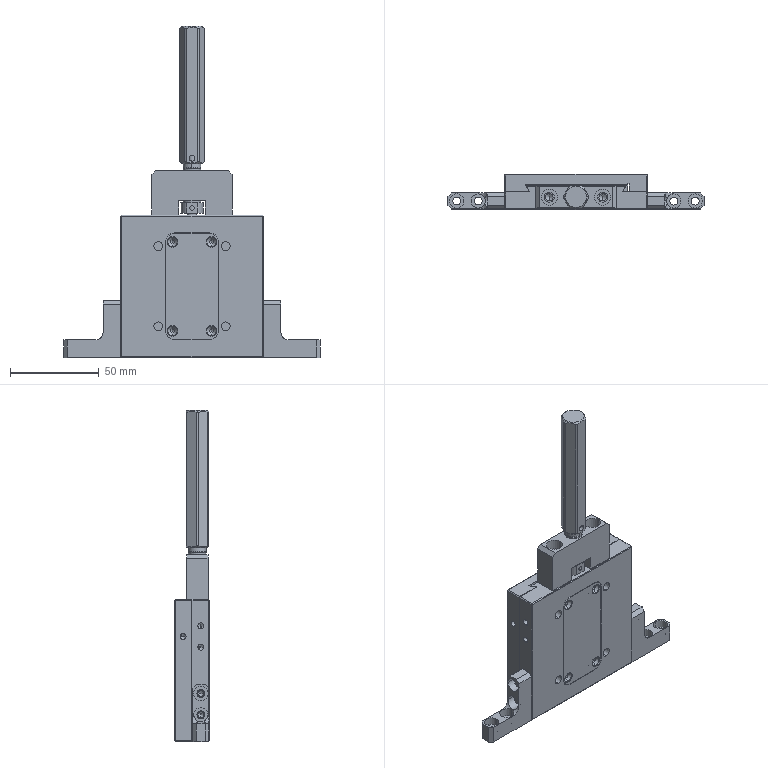Part | SolidWorks | features BaseBody 1 | 1 solid | 537 faces | box 144 x 20 x 186 mm | volume 140679 mm3 | cylinder 259 | plane 170 | cone 108 | commonest cylinder face diameters 3.3 x80 8 x36 4.5 x24 5 x18 6 x16 10 x14